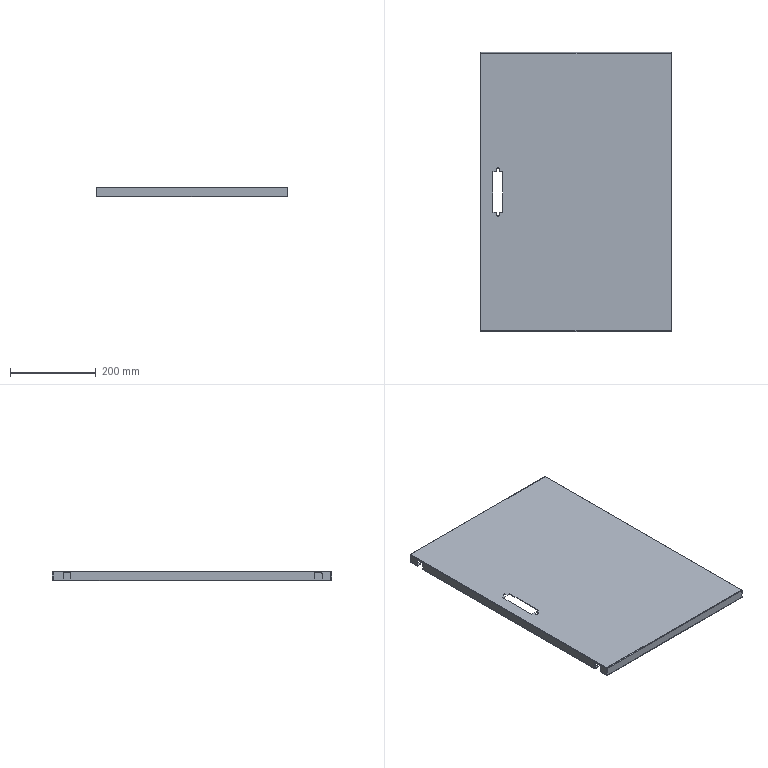Part | SolidWorks | features ICE 3, EdgeFlange 2, FlatPattern 1, LPattern 1, SMBaseFlange 1, SheetMetal 1 | 1 solid | 118 faces | box 447 x 650 x 22 mm | volume 527115 mm3 | plane 76 | cylinder 26 | spline 16 | commonest cylinder face diameters 0.2 x10 3.2 x10 4 x4 7 x2